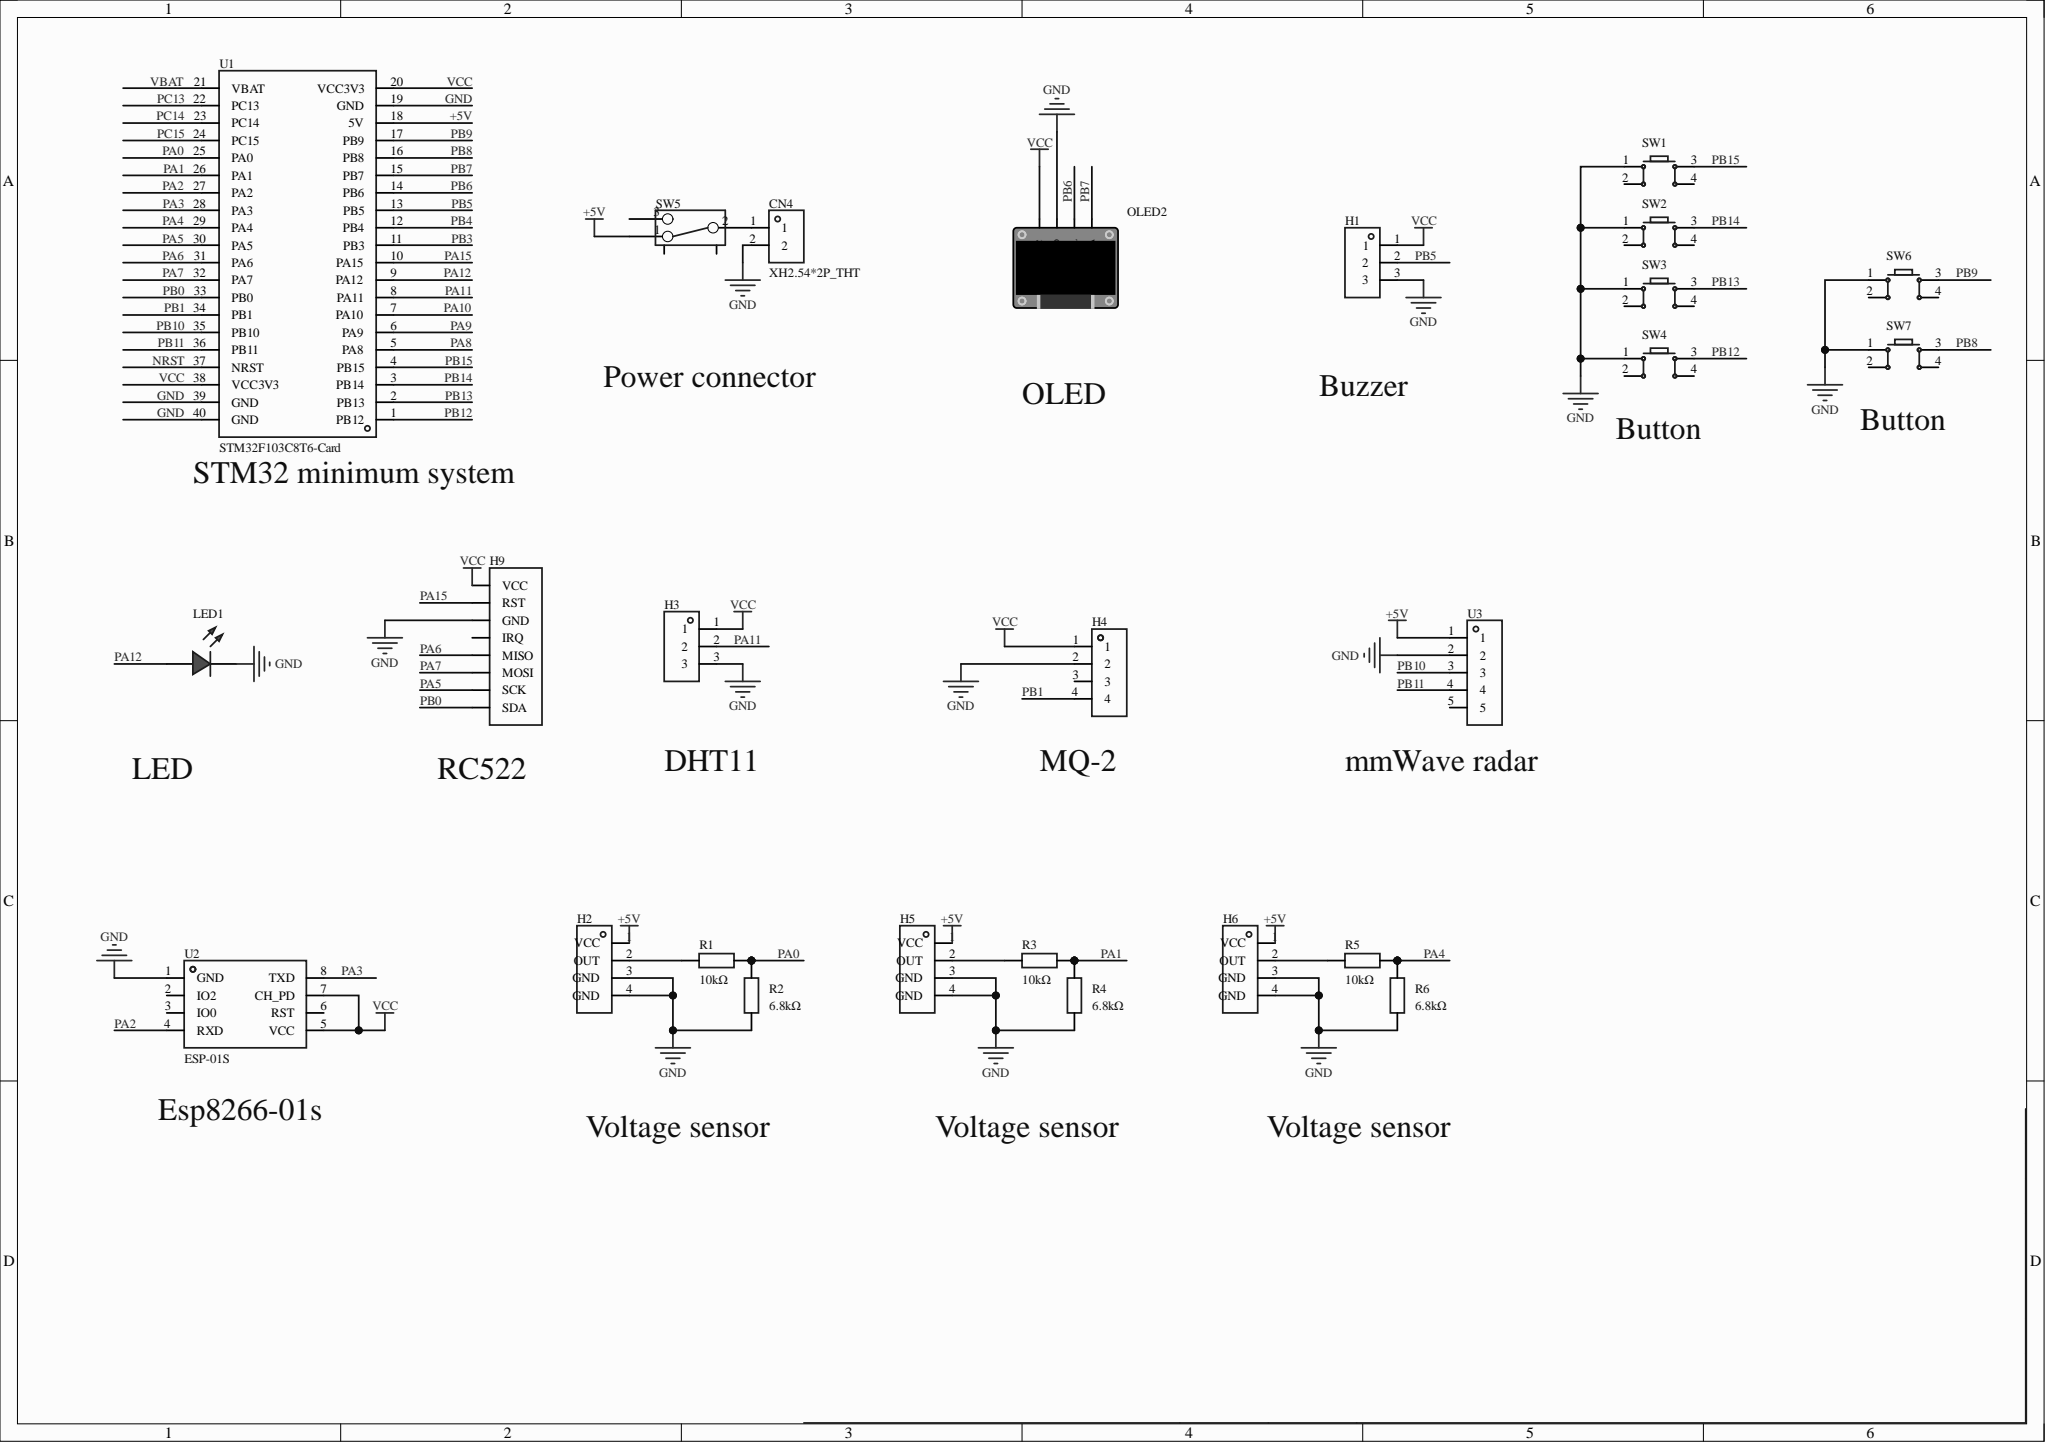Circuit board | Altium Designer | 26 parts | 31 nets
Bill of materials:
Comment,Description,Designator,Footprint,LibRef,Quantity
"XH2.54*2P_THT","","CN4","CONN-TH_2P-P2.50-XH2.54-2P","XH2.54*2P_直插","1"
"","","H1, H3","HDR-TH_3P-P2.54-V-F","HDR-F_2.54_1x3P","2"
"","","H2, H4, H5, H6","HDR-TH_4P-P2.54-V-F","HDR-F_2.54_1x4P","4"
"","","H9","HDR-TH_8P-P2.54-V-F-1","HDR-F_2.54_1x8P","1"
"","","LED1","LED_TH-3mm","LED_TH-R_3mm","1"
"","","OLED2","0.96OLED_4P","0.96OLED模块_4P","1"
"10kΩ","","R1, R3, R5","Res_1/8W","Res_AXIAL-1/8W","3"
"6.8kΩ","","R2, R4, R6","Res_1/8W","Res_AXIAL-1/8W","3"
"","","SW1, SW2, SW3, SW4, SW6, SW7","SW-TH_4P-L6.0-W6.0-P4.50-LS6.5","Key_TH_6x6x6","6"
"","","SW5","拨动开关","拨动开关_正","1"
"STM32F103C8T6-Card","","U1","CONN-TH_L53.3-W22.9_STM32F103C8T6-CARD","STM32F103C8T6-Card","1"
"ESP-01S","","U2","WIFIM-TH_ESP-01S","ESP-01S_C111009","1"
"FPH12728-S05S1014190140B","","U3","HDR-TH_5P-P1.27-V-M-1","FPH12728-S05S1014190140B","1"
Netlist (Protel format):
[
CN4
CONN-TH_2P-P2.50-XH2.54-2P
XH2.54*2P_THT



]
[
H1
HDR-TH_3P-P2.54-V-F




]
[
H2
HDR-TH_4P-P2.54-V-F




]
[
H3
HDR-TH_3P-P2.54-V-F




]
[
H4
HDR-TH_4P-P2.54-V-F




]
[
H5
HDR-TH_4P-P2.54-V-F




]
[
H6
HDR-TH_4P-P2.54-V-F




]
[
H9
HDR-TH_8P-P2.54-V-F-1




]
[
LED1
LED_TH-3mm




]
[
OLED2
0.96OLED_4P




]
[
R1
Res_1/8W
10kΩ



]
[
R2
Res_1/8W
6.8kΩ



]
[
R3
Res_1/8W
10kΩ



]
[
R4
Res_1/8W
6.8kΩ



]
[
R5
Res_1/8W
10kΩ



]
[
R6
Res_1/8W
6.8kΩ



]
[
SW1
SW-TH_4P-L6.0-W6.0-P4.50-LS6.5




]
[
SW2
SW-TH_4P-L6.0-W6.0-P4.50-LS6.5




]
[
SW3
SW-TH_4P-L6.0-W6.0-P4.50-LS6.5




]
[
SW4
SW-TH_4P-L6.0-W6.0-P4.50-LS6.5




]
[
SW5
拨动开关




]
[
SW6
SW-TH_4P-L6.0-W6.0-P4.50-LS6.5




]
[
SW7
SW-TH_4P-L6.0-W6.0-P4.50-LS6.5




]
[
U1
CONN-TH_L53.3-W22.9_STM32F103C8T6-CARD
STM32F103C8T6-Card



]
[
U2
WIFIM-TH_ESP-01S
ESP-01S



]
[
U3
HDR-TH_5P-P1.27-V-M-1
FPH12728-S05S1014190140B



]
(
VCC
H1-1
H3-1
H4-1
H9-1
OLED2-1
U1-20
U1-38
U2-5
U2-7
)
(
PB15
SW1-3
U1-4
)
(
PB14
SW2-3
U1-3
)
(
PB13
SW3-3
U1-2
)
(
PB12
SW4-3
U1-1
)
(
PB11
U1-36
U3-4
)
(
PB10
U1-35
U3-3
)
(
PB9
SW6-3
U1-17
)
(
PB8
SW7-3
U1-16
)
(
PB7
OLED2-4
U1-15
)
(
PB6
OLED2-3
U1-14
)
(
PB5
H1-2
U1-13
)
(
PB1
H4-4
U1-34
)
(
PB0
H9-8
U1-33
)
(
PA15
H9-2
U1-10
)
(
PA12
LED1-1
U1-9
)
(
PA11
H3-2
U1-8
)
(
PA7
H9-6
U1-32
)
(
PA6
H9-5
U1-31
)
(
PA5
H9-7
U1-30
)
(
PA4
R5-2
R6-2
U1-29
)
(
PA3
U1-28
U2-8
)
(
PA2
U1-27
U2-4
)
(
PA1
R3-2
R4-2
U1-26
)
(
PA0
R1-2
R2-2
U1-25
)
(
NetH6_2
H6-2
R5-1
)
(
NetH5_2
H5-2
R3-1
)
(
NetH2_2
H2-2
R1-1
)
(
NetCN4_1
CN4-1
SW5-2
)
(
GND
CN4-2
H1-3
H2-3
H2-4
H3-3
H4-2
H5-3
H5-4
H6-3
H6-4
H9-3
LED1-2
OLED2-2
R2-1
R4-1
R6-1
SW1-1
SW2-1
SW3-1
SW4-1
SW6-1
SW7-1
U1-19
U1-39
U1-40
U2-1
U3-2
)
(
+5V
H2-1
H5-1
H6-1
SW5-1
U1-18
U3-1
)